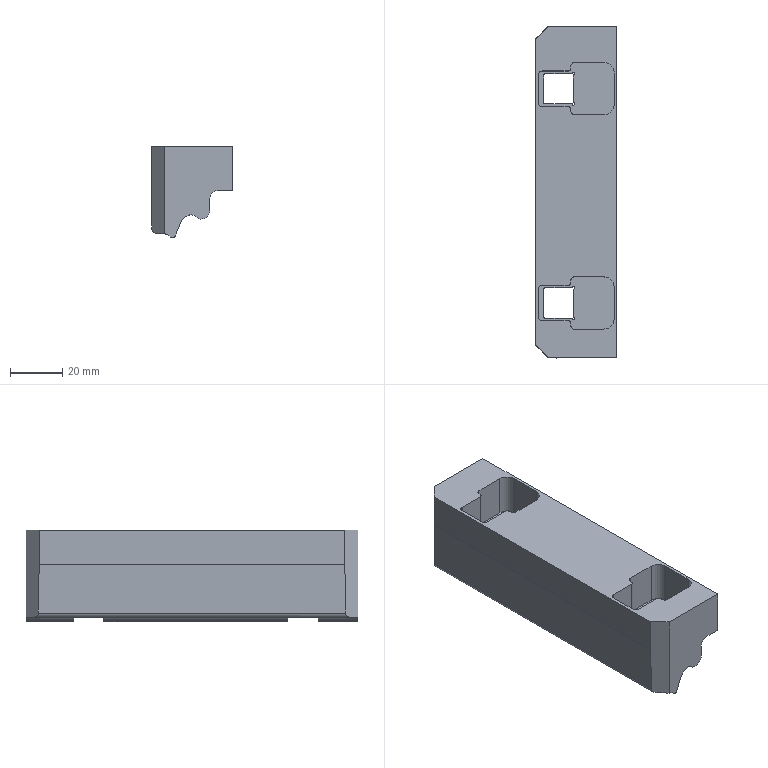Part | 1 solid | 77 faces | box 31.262 x 127 x 35.026 mm | volume 84488 mm3 | plane 43 | cylinder 34 | commonest cylinder face diameters 1 x8 3 x8 2 x4 8 x4 2.085 x3 11.296 x3